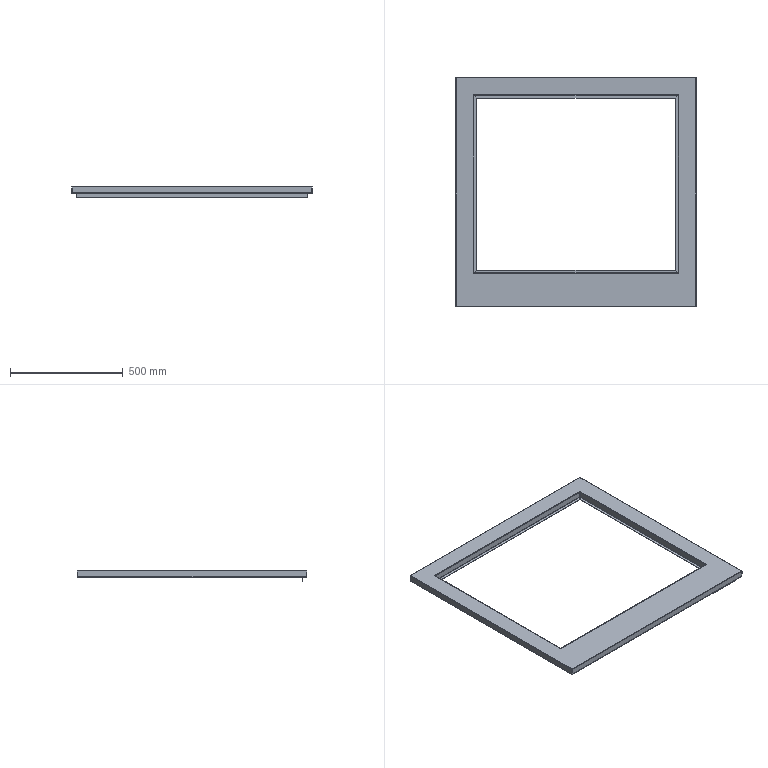Part | SolidWorks | features EdgeFlange 5, FlatPattern 1, HoleWzd 1, ICE 1, SMBaseFlange 1, SheetMetal 1 | 1 solid | 160 faces | box 1070 x 1020 x 48.5 mm | volume 1078277 mm3 | plane 86 | cylinder 42 | spline 32 | commonest cylinder face diameters 1 x17 4 x17 5 x8